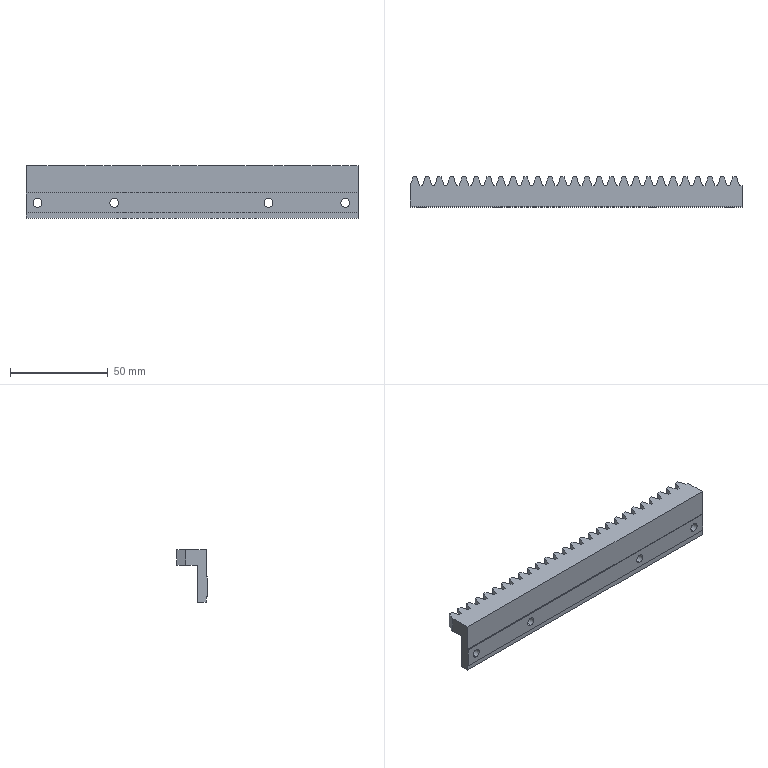Part | SolidWorks | features ICE 4, LPattern 3, Boss 1, Chamfer 1, Extrusion 1, Fillet 1 | 1 solid | 127 faces | box 169.646 x 15.5 x 27 mm | volume 32516 mm3 | plane 119 | cylinder 8 | commonest cylinder face diameters 4.5 x8